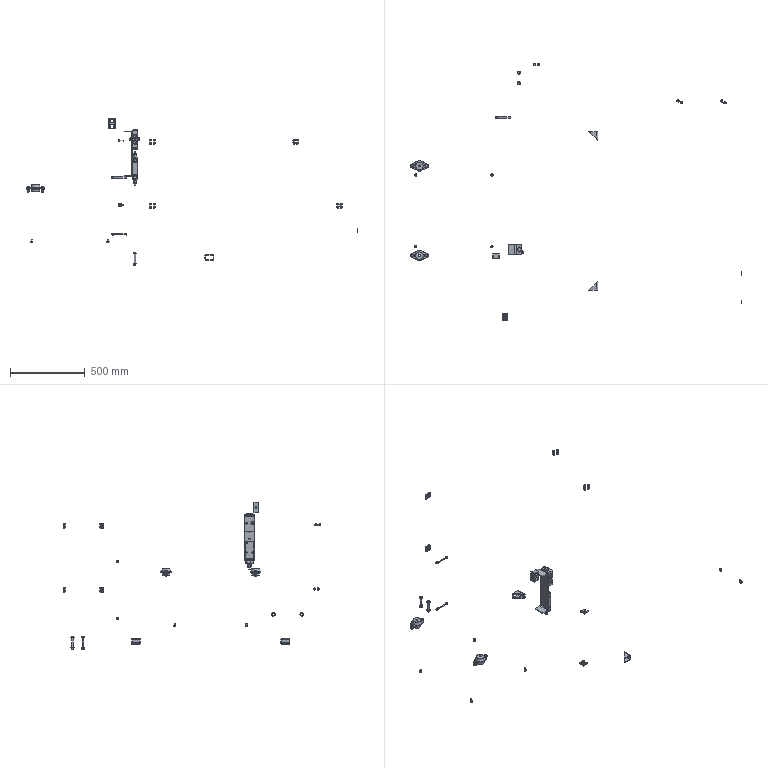Part | STEP file | COMPOUND | 123 solids | 2213 faces | box 2217 x 1725 x 986 mm | volume 1142087 mm3 | plane 1058 | cone 436 | other 374 | cylinder 319 | torus 26 | commonest cylinder face diameters 8.4 x30 15 x30 21 x22 10 x21 8 x19 8.1 x16